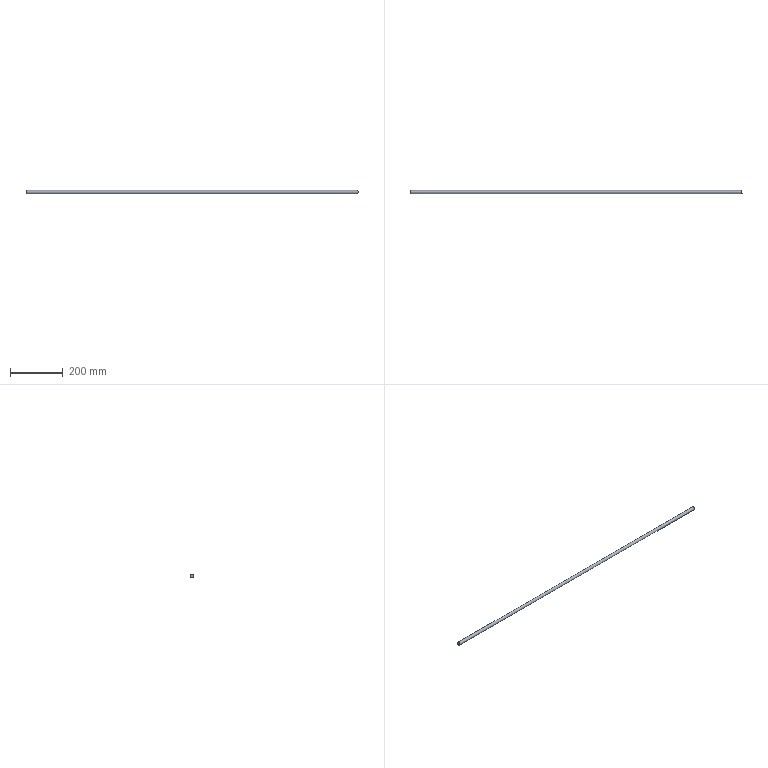Part | STEP file | solid 22 | 1 solid | 3 faces | box 1260 x 12 x 12 mm | volume 142503 mm3 | plane 2 | cylinder 1 | commonest cylinder face diameters 12 x1